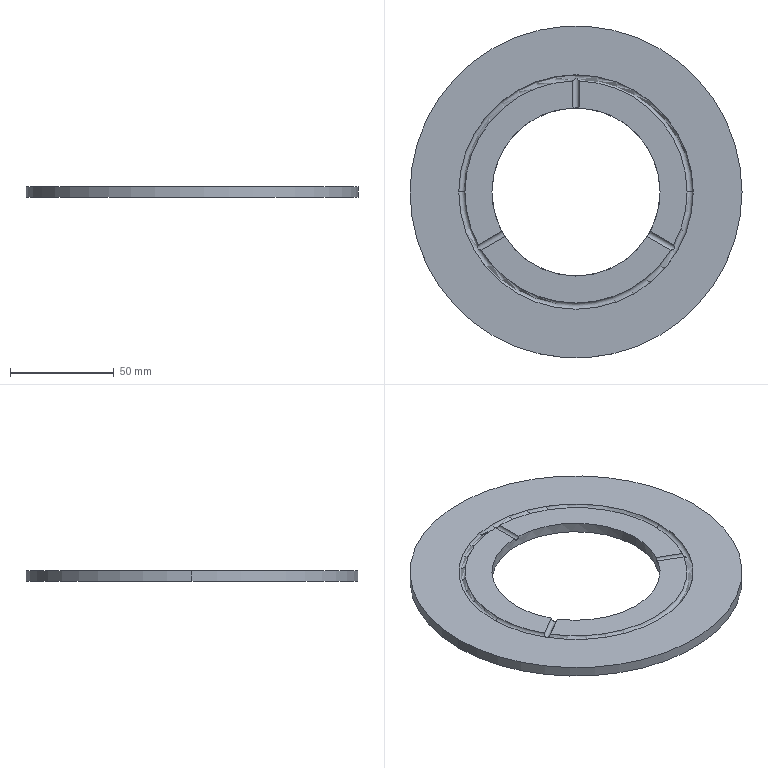Part | SolidWorks | features CirPattern 1, Extrusion 1, ICE 1, SweepCut 1 | 1 solid | 15 faces | box 160 x 160 x 5 mm | volume 73404 mm3 | cylinder 8 | plane 5 | torus 2 | commonest cylinder face diameters 3 x4 81 x2 160 x2
STEP:
#1=CARTESIAN_POINT('',(0.,55.,3.5));
#2=VERTEX_POINT('',#1);
#3=CARTESIAN_POINT('',(1.5,53.479,5.));
#4=VERTEX_POINT('',#3);
#5=CARTESIAN_POINT('',(0.,55.,3.5));
#6=CARTESIAN_POINT('',(0.08396,54.916,3.5));
#7=CARTESIAN_POINT('',(0.1693,54.83,3.507));
#8=CARTESIAN_POINT('',(0.3359,54.663,3.536));
#9=CARTESIAN_POINT('',(0.4182,54.58,3.557));
#10=CARTESIAN_POINT('',(0.6622,54.334,3.643));
#11=CARTESIAN_POINT('',(0.8218,54.172,3.731));
#12=CARTESIAN_POINT('',(1.11,53.879,3.974));
#13=CARTESIAN_POINT('',(1.242,53.744,4.131));
#14=CARTESIAN_POINT('',(1.39,53.592,4.425));
#15=CARTESIAN_POINT('',(1.43,53.551,4.531));
#16=CARTESIAN_POINT('',(1.485,53.494,4.758));
#17=CARTESIAN_POINT('',(1.5,53.479,4.878));
#18=CARTESIAN_POINT('',(1.5,53.479,5.));
#19=B_SPLINE_CURVE_WITH_KNOTS('',3,(#5,#6,#7,#8,#9,#10,#11,#12,#13,#14,#15,#16,#17,#18),.UNSPECIFIED.,.F.,.F.,(4,2,2,2,2,2,4),(-0.000007746,0.0003485,0.0007047,0.001417,0.00213,0.002486,0.002842),.UNSPECIFIED.);
#20=EDGE_CURVE('',#2,#4,#19,.T.);
#21=ORIENTED_EDGE('',*,*,#20,.F.);
#22=CARTESIAN_POINT('',(0.,40.5,3.5));
#23=VERTEX_POINT('',#22);
#24=CARTESIAN_POINT('',(0.,55.,3.5));
#25=DIRECTION('',(0.,-1.,0.));
#26=VECTOR('',#25,1000.);
#27=LINE('',#24,#26);
#28=EDGE_CURVE('',#2,#23,#27,.T.);
#29=ORIENTED_EDGE('',*,*,#28,.T.);
#30=CARTESIAN_POINT('',(1.5,40.472,5.));
#31=VERTEX_POINT('',#30);
#32=CARTESIAN_POINT('',(1.5,40.472,5.));
#33=CARTESIAN_POINT('',(1.5,40.472,4.901));
#34=CARTESIAN_POINT('',(1.49,40.473,4.803));
#35=CARTESIAN_POINT('',(1.452,40.474,4.612));
#36=CARTESIAN_POINT('',(1.423,40.475,4.516));
#37=CARTESIAN_POINT('',(1.348,40.478,4.335));
#38=CARTESIAN_POINT('',(1.302,40.479,4.248));
#39=CARTESIAN_POINT('',(1.193,40.482,4.085));
#40=CARTESIAN_POINT('',(1.13,40.484,4.008));
#41=CARTESIAN_POINT('',(0.9218,40.49,3.801));
#42=CARTESIAN_POINT('',(0.7544,40.493,3.689));
#43=CARTESIAN_POINT('',(0.3932,40.498,3.539));
#44=CARTESIAN_POINT('',(0.1957,40.5,3.5));
#45=CARTESIAN_POINT('',(0.,40.5,3.5));
#46=B_SPLINE_CURVE_WITH_KNOTS('',3,(#32,#33,#34,#35,#36,#37,#38,#39,#40,#41,#42,#43,#44,#45),.UNSPECIFIED.,.F.,.F.,(4,2,2,2,2,2,4),(0.,0.0002932,0.0005864,0.0008796,0.001173,0.001759,0.002346),.UNSPECIFIED.);
#47=EDGE_CURVE('',#31,#23,#46,.T.);
#48=ORIENTED_EDGE('',*,*,#47,.F.);
#49=CARTESIAN_POINT('',(1.5,55.,5.));
#50=DIRECTION('',(0.,-1.,0.));
#51=VECTOR('',#50,1000.);
#52=LINE('',#49,#51);
#53=EDGE_CURVE('',#4,#31,#52,.T.);
#54=ORIENTED_EDGE('',*,*,#53,.F.);
#55=EDGE_LOOP('',(#21,#29,#48,#54));
#56=FACE_OUTER_BOUND('',#55,.T.);
#57=CARTESIAN_POINT('',(0.,55.,5.));
#58=DIRECTION('',(0.,-1.,0.));
#59=DIRECTION('',(0.,0.,-1.));
#60=AXIS2_PLACEMENT_3D('',#57,#58,#59);
#61=CYLINDRICAL_SURFACE('',#60,1.5);
#62=ADVANCED_FACE('',(#56),#61,.F.);
#63=CARTESIAN_POINT('',(80.,0.,5.));
#64=VERTEX_POINT('',#63);
#65=CARTESIAN_POINT('',(-80.,0.,5.));
#66=VERTEX_POINT('',#65);
#67=CARTESIAN_POINT('',(0.,0.,5.));
#68=DIRECTION('',(0.,0.,1.));
#69=DIRECTION('',(1.,0.,0.));
#70=AXIS2_PLACEMENT_3D('',#67,#68,#69);
#71=CIRCLE('',#70,80.);
#72=EDGE_CURVE('',#64,#66,#71,.T.);
#73=ORIENTED_EDGE('',*,*,#72,.F.);
#74=CARTESIAN_POINT('',(80.,0.,0.));
#75=VERTEX_POINT('',#74);
#76=CARTESIAN_POINT('',(80.,0.,5.));
#77=DIRECTION('',(0.,0.,-1.));
#78=VECTOR('',#77,1000.);
#79=LINE('',#76,#78);
#80=EDGE_CURVE('',#64,#75,#79,.T.);
#81=ORIENTED_EDGE('',*,*,#80,.T.);
#82=CARTESIAN_POINT('',(-80.,0.,0.));
#83=VERTEX_POINT('',#82);
#84=CARTESIAN_POINT('',(0.,0.,0.));
#85=DIRECTION('',(0.,0.,1.));
#86=DIRECTION('',(1.,0.,0.));
#87=AXIS2_PLACEMENT_3D('',#84,#85,#86);
#88=CIRCLE('',#87,80.);
#89=EDGE_CURVE('',#75,#83,#88,.T.);
#90=ORIENTED_EDGE('',*,*,#89,.T.);
#91=CARTESIAN_POINT('',(-80.,0.,5.));
#92=DIRECTION('',(0.,0.,-1.));
#93=VECTOR('',#92,1000.);
#94=LINE('',#91,#93);
#95=EDGE_CURVE('',#66,#83,#94,.T.);
#96=ORIENTED_EDGE('',*,*,#95,.F.);
#97=EDGE_LOOP('',(#73,#81,#90,#96));
#98=FACE_OUTER_BOUND('',#97,.T.);
#99=CARTESIAN_POINT('',(0.,0.,5.));
#100=DIRECTION('',(0.,0.,-1.));
#101=DIRECTION('',(-1.,0.,0.));
#102=AXIS2_PLACEMENT_3D('',#99,#100,#101);
#103=CYLINDRICAL_SURFACE('',#102,80.);
#104=ADVANCED_FACE('',(#98),#103,.T.);
#105=CARTESIAN_POINT('',(-53.5,0.,5.));
#106=VERTEX_POINT('',#105);
#107=CARTESIAN_POINT('',(-47.064,-25.44,5.));
#108=VERTEX_POINT('',#107);
#109=CARTESIAN_POINT('',(0.,0.,5.));
#110=DIRECTION('',(0.,0.,1.));
#111=DIRECTION('',(-1.,0.,0.));
#112=AXIS2_PLACEMENT_3D('',#109,#110,#111);
#113=CIRCLE('',#112,53.5);
#114=EDGE_CURVE('',#106,#108,#113,.T.);
#115=ORIENTED_EDGE('',*,*,#114,.F.);
#116=CARTESIAN_POINT('',(-56.5,0.,5.));
#117=VERTEX_POINT('',#116);
#118=CARTESIAN_POINT('',(-55.,0.,5.));
#119=DIRECTION('',(0.,1.,0.));
#120=DIRECTION('',(-1.,0.,0.));
#121=AXIS2_PLACEMENT_3D('',#118,#119,#120);
#122=CIRCLE('',#121,1.5);
#123=EDGE_CURVE('',#106,#117,#122,.T.);
#124=ORIENTED_EDGE('',*,*,#123,.T.);
#125=CARTESIAN_POINT('',(56.5,0.,5.));
#126=VERTEX_POINT('',#125);
#127=CARTESIAN_POINT('',(0.,0.,5.));
#128=DIRECTION('',(0.,0.,-1.));
#129=DIRECTION('',(1.,0.,0.));
#130=AXIS2_PLACEMENT_3D('',#127,#128,#129);
#131=CIRCLE('',#130,56.5);
#132=EDGE_CURVE('',#126,#117,#131,.T.);
#133=ORIENTED_EDGE('',*,*,#132,.F.);
#134=CARTESIAN_POINT('',(53.5,0.,5.));
#135=VERTEX_POINT('',#134);
#136=CARTESIAN_POINT('',(55.,0.,5.));
#137=DIRECTION('',(0.,-1.,0.));
#138=DIRECTION('',(0.,0.,-1.));
#139=AXIS2_PLACEMENT_3D('',#136,#137,#138);
#140=CIRCLE('',#139,1.5);
#141=EDGE_CURVE('',#135,#126,#140,.T.);
#142=ORIENTED_EDGE('',*,*,#141,.F.);
#143=CARTESIAN_POINT('',(47.064,-25.44,5.));
#144=VERTEX_POINT('',#143);
#145=CARTESIAN_POINT('',(0.,0.,5.));
#146=DIRECTION('',(0.,0.,1.));
#147=DIRECTION('',(-1.,0.,0.));
#148=AXIS2_PLACEMENT_3D('',#145,#146,#147);
#149=CIRCLE('',#148,53.5);
#150=EDGE_CURVE('',#144,#135,#149,.T.);
#151=ORIENTED_EDGE('',*,*,#150,.F.);
#152=CARTESIAN_POINT('',(47.631,-27.5,3.5));
#153=VERTEX_POINT('',#152);
#154=CARTESIAN_POINT('',(47.064,-25.44,5.));
#155=CARTESIAN_POINT('',(47.064,-25.44,4.757));
#156=CARTESIAN_POINT('',(47.088,-25.524,4.524));
#157=CARTESIAN_POINT('',(47.164,-25.794,4.133));
#158=CARTESIAN_POINT('',(47.215,-25.975,3.976));
#159=CARTESIAN_POINT('',(47.325,-26.373,3.731));
#160=CARTESIAN_POINT('',(47.384,-26.587,3.645));
#161=CARTESIAN_POINT('',(47.507,-27.038,3.528));
#162=CARTESIAN_POINT('',(47.57,-27.269,3.5));
#163=CARTESIAN_POINT('',(47.631,-27.5,3.5));
#164=B_SPLINE_CURVE_WITH_KNOTS('',3,(#154,#155,#156,#157,#158,#159,#160,#161,#162,#163),.UNSPECIFIED.,.F.,.F.,(4,2,2,2,4),(0.000000196,0.0007165,0.001433,0.002149,0.002865),.UNSPECIFIED.);
#165=EDGE_CURVE('',#144,#153,#164,.T.);
#166=ORIENTED_EDGE('',*,*,#165,.T.);
#167=CARTESIAN_POINT('',(45.564,-28.039,5.));
#168=VERTEX_POINT('',#167);
#169=CARTESIAN_POINT('',(47.631,-27.5,3.5));
#170=CARTESIAN_POINT('',(47.517,-27.531,3.5));
#171=CARTESIAN_POINT('',(47.4,-27.562,3.507));
#172=CARTESIAN_POINT('',(47.172,-27.622,3.536));
#173=CARTESIAN_POINT('',(47.059,-27.652,3.557));
#174=CARTESIAN_POINT('',(46.724,-27.74,3.643));
#175=CARTESIAN_POINT('',(46.504,-27.798,3.731));
#176=CARTESIAN_POINT('',(46.105,-27.901,3.974));
#177=CARTESIAN_POINT('',(45.923,-27.947,4.131));
#178=CARTESIAN_POINT('',(45.718,-28.,4.425));
#179=CARTESIAN_POINT('',(45.662,-28.014,4.531));
#180=CARTESIAN_POINT('',(45.585,-28.033,4.758));
#181=CARTESIAN_POINT('',(45.564,-28.039,4.878));
#182=CARTESIAN_POINT('',(45.564,-28.039,5.));
#183=B_SPLINE_CURVE_WITH_KNOTS('',3,(#169,#170,#171,#172,#173,#174,#175,#176,#177,#178,#179,#180,#181,#182),.UNSPECIFIED.,.F.,.F.,(4,2,2,2,2,2,4),(-0.000007746,0.0003485,0.0007047,0.001417,0.00213,0.002486,0.002842),.UNSPECIFIED.);
#184=EDGE_CURVE('',#153,#168,#183,.T.);
#185=ORIENTED_EDGE('',*,*,#184,.T.);
#186=CARTESIAN_POINT('',(-45.564,-28.039,5.));
#187=VERTEX_POINT('',#186);
#188=CARTESIAN_POINT('',(0.,0.,5.));
#189=DIRECTION('',(0.,0.,1.));
#190=DIRECTION('',(-1.,0.,0.));
#191=AXIS2_PLACEMENT_3D('',#188,#189,#190);
#192=CIRCLE('',#191,53.5);
#193=EDGE_CURVE('',#187,#168,#192,.T.);
#194=ORIENTED_EDGE('',*,*,#193,.F.);
#195=CARTESIAN_POINT('',(-47.631,-27.5,3.5));
#196=VERTEX_POINT('',#195);
#197=CARTESIAN_POINT('',(-45.564,-28.039,5.));
#198=CARTESIAN_POINT('',(-45.564,-28.039,4.757));
#199=CARTESIAN_POINT('',(-45.649,-28.017,4.524));
#200=CARTESIAN_POINT('',(-45.921,-27.948,4.133));
#201=CARTESIAN_POINT('',(-46.102,-27.901,3.976));
#202=CARTESIAN_POINT('',(-46.503,-27.798,3.731));
#203=CARTESIAN_POINT('',(-46.717,-27.742,3.645));
#204=CARTESIAN_POINT('',(-47.169,-27.623,3.528));
#205=CARTESIAN_POINT('',(-47.401,-27.562,3.5));
#206=CARTESIAN_POINT('',(-47.631,-27.5,3.5));
#207=B_SPLINE_CURVE_WITH_KNOTS('',3,(#197,#198,#199,#200,#201,#202,#203,#204,#205,#206),.UNSPECIFIED.,.F.,.F.,(4,2,2,2,4),(0.000000196,0.0007165,0.001433,0.002149,0.002865),.UNSPECIFIED.);
#208=EDGE_CURVE('',#187,#196,#207,.T.);
#209=ORIENTED_EDGE('',*,*,#208,.T.);
#210=CARTESIAN_POINT('',(-47.631,-27.5,3.5));
#211=CARTESIAN_POINT('',(-47.601,-27.385,3.5));
#212=CARTESIAN_POINT('',(-47.569,-27.269,3.507));
#213=CARTESIAN_POINT('',(-47.508,-27.041,3.536));
#214=CARTESIAN_POINT('',(-47.477,-26.928,3.557));
#215=CARTESIAN_POINT('',(-47.386,-26.594,3.643));
#216=CARTESIAN_POINT('',(-47.325,-26.374,3.731));
#217=CARTESIAN_POINT('',(-47.215,-25.978,3.974));
#218=CARTESIAN_POINT('',(-47.165,-25.797,4.131));
#219=CARTESIAN_POINT('',(-47.107,-25.593,4.425));
#220=CARTESIAN_POINT('',(-47.092,-25.538,4.531));
#221=CARTESIAN_POINT('',(-47.07,-25.461,4.758));
#222=CARTESIAN_POINT('',(-47.064,-25.44,4.878));
#223=CARTESIAN_POINT('',(-47.064,-25.44,5.));
#224=B_SPLINE_CURVE_WITH_KNOTS('',3,(#210,#211,#212,#213,#214,#215,#216,#217,#218,#219,#220,#221,#222,#223),.UNSPECIFIED.,.F.,.F.,(4,2,2,2,2,2,4),(-0.000007746,0.0003485,0.0007047,0.001417,0.00213,0.002486,0.002842),.UNSPECIFIED.);
#225=EDGE_CURVE('',#196,#108,#224,.T.);
#226=ORIENTED_EDGE('',*,*,#225,.T.);
#227=EDGE_LOOP('',(#115,#124,#133,#142,#151,#166,#185,#194,#209,#226));
#228=FACE_OUTER_BOUND('',#227,.T.);
#229=CARTESIAN_POINT('',(0.,0.,5.));
#230=DIRECTION('',(0.,0.,1.));
#231=DIRECTION('',(1.,0.,0.));
#232=AXIS2_PLACEMENT_3D('',#229,#230,#231);
#233=TOROIDAL_SURFACE('',#232,55.,1.5);
#234=ADVANCED_FACE('',(#228),#233,.F.);
#235=CARTESIAN_POINT('',(35.8,-18.937,5.));
#236=VERTEX_POINT('',#235);
#237=CARTESIAN_POINT('',(40.5,0.,5.));
#238=VERTEX_POINT('',#237);
#239=CARTESIAN_POINT('',(0.,0.,5.));
#240=DIRECTION('',(0.,0.,1.));
#241=DIRECTION('',(1.,0.,0.));
#242=AXIS2_PLACEMENT_3D('',#239,#240,#241);
#243=CIRCLE('',#242,40.5);
#244=EDGE_CURVE('',#236,#238,#243,.T.);
#245=ORIENTED_EDGE('',*,*,#244,.T.);
#246=CARTESIAN_POINT('',(40.5,0.,0.));
#247=VERTEX_POINT('',#246);
#248=CARTESIAN_POINT('',(40.5,0.,5.));
#249=DIRECTION('',(0.,0.,-1.));
#250=VECTOR('',#249,1000.);
#251=LINE('',#248,#250);
#252=EDGE_CURVE('',#238,#247,#251,.T.);
#253=ORIENTED_EDGE('',*,*,#252,.T.);
#254=CARTESIAN_POINT('',(-40.5,0.,0.));
#255=VERTEX_POINT('',#254);
#256=CARTESIAN_POINT('',(0.,0.,0.));
#257=DIRECTION('',(0.,0.,1.));
#258=DIRECTION('',(1.,0.,0.));
#259=AXIS2_PLACEMENT_3D('',#256,#257,#258);
#260=CIRCLE('',#259,40.5);
#261=EDGE_CURVE('',#255,#247,#260,.T.);
#262=ORIENTED_EDGE('',*,*,#261,.F.);
#263=CARTESIAN_POINT('',(-40.5,0.,5.));
#264=VERTEX_POINT('',#263);
#265=CARTESIAN_POINT('',(-40.5,0.,5.));
#266=DIRECTION('',(0.,0.,-1.));
#267=VECTOR('',#266,1000.);
#268=LINE('',#265,#267);
#269=EDGE_CURVE('',#264,#255,#268,.T.);
#270=ORIENTED_EDGE('',*,*,#269,.F.);
#271=CARTESIAN_POINT('',(-35.8,-18.937,5.));
#272=VERTEX_POINT('',#271);
#273=CARTESIAN_POINT('',(0.,0.,5.));
#274=DIRECTION('',(0.,0.,1.));
#275=DIRECTION('',(1.,0.,0.));
#276=AXIS2_PLACEMENT_3D('',#273,#274,#275);
#277=CIRCLE('',#276,40.5);
#278=EDGE_CURVE('',#264,#272,#277,.T.);
#279=ORIENTED_EDGE('',*,*,#278,.T.);
#280=CARTESIAN_POINT('',(-34.3,-21.535,5.));
#281=VERTEX_POINT('',#280);
#282=CARTESIAN_POINT('',(-35.8,-18.937,5.));
#283=CARTESIAN_POINT('',(-35.8,-18.937,4.901));
#284=CARTESIAN_POINT('',(-35.795,-18.946,4.803));
#285=CARTESIAN_POINT('',(-35.778,-18.979,4.612));
#286=CARTESIAN_POINT('',(-35.764,-19.005,4.516));
#287=CARTESIAN_POINT('',(-35.729,-19.071,4.335));
#288=CARTESIAN_POINT('',(-35.707,-19.112,4.249));
#289=CARTESIAN_POINT('',(-35.655,-19.208,4.086));
#290=CARTESIAN_POINT('',(-35.625,-19.264,4.008));
#291=CARTESIAN_POINT('',(-35.526,-19.446,3.801));
#292=CARTESIAN_POINT('',(-35.446,-19.593,3.689));
#293=CARTESIAN_POINT('',(-35.27,-19.908,3.539));
#294=CARTESIAN_POINT('',(-35.172,-20.08,3.5));
#295=CARTESIAN_POINT('',(-35.025,-20.334,3.5));
#296=CARTESIAN_POINT('',(-34.975,-20.42,3.51));
#297=CARTESIAN_POINT('',(-34.878,-20.586,3.548));
#298=CARTESIAN_POINT('',(-34.83,-20.667,3.576));
#299=CARTESIAN_POINT('',(-34.737,-20.823,3.651));
#300=CARTESIAN_POINT('',(-34.692,-20.898,3.698));
#301=CARTESIAN_POINT('',(-34.608,-21.037,3.807));
#302=CARTESIAN_POINT('',(-34.568,-21.102,3.869));
#303=CARTESIAN_POINT('',(-34.459,-21.281,4.079));
#304=CARTESIAN_POINT('',(-34.4,-21.374,4.244));
#305=CARTESIAN_POINT('',(-34.341,-21.47,4.517));
#306=CARTESIAN_POINT('',(-34.326,-21.494,4.61));
#307=CARTESIAN_POINT('',(-34.305,-21.527,4.803));
#308=CARTESIAN_POINT('',(-34.3,-21.535,4.902));
#309=CARTESIAN_POINT('',(-34.3,-21.535,5.));
#310=B_SPLINE_CURVE_WITH_KNOTS('',3,(#282,#283,#284,#285,#286,#287,#288,#289,#290,#291,#292,#293,#294,#295,#296,#297,#298,#299,#300,#301,#302,#303,#304,#305,#306,#307,#308,#309),.UNSPECIFIED.,.F.,.F.,(4,2,2,2,2,2,2,2,2,2,2,2,2,4),(0.,0.0002931,0.0005863,0.0008794,0.001173,0.001759,0.002345,0.002638,0.002931,0.003224,0.003518,0.004104,0.004397,0.00469),.UNSPECIFIED.);
#311=EDGE_CURVE('',#272,#281,#310,.T.);
#312=ORIENTED_EDGE('',*,*,#311,.T.);
#313=CARTESIAN_POINT('',(34.3,-21.535,5.));
#314=VERTEX_POINT('',#313);
#315=CARTESIAN_POINT('',(0.,0.,5.));
#316=DIRECTION('',(0.,0.,1.));
#317=DIRECTION('',(1.,0.,0.));
#318=AXIS2_PLACEMENT_3D('',#315,#316,#317);
#319=CIRCLE('',#318,40.5);
#320=EDGE_CURVE('',#281,#314,#319,.T.);
#321=ORIENTED_EDGE('',*,*,#320,.T.);
#322=CARTESIAN_POINT('',(34.3,-21.535,5.));
#323=CARTESIAN_POINT('',(34.3,-21.535,4.901));
#324=CARTESIAN_POINT('',(34.305,-21.527,4.803));
#325=CARTESIAN_POINT('',(34.325,-21.495,4.612));
#326=CARTESIAN_POINT('',(34.341,-21.47,4.516));
#327=CARTESIAN_POINT('',(34.381,-21.406,4.335));
#328=CARTESIAN_POINT('',(34.405,-21.367,4.249));
#329=CARTESIAN_POINT('',(34.462,-21.274,4.086));
#330=CARTESIAN_POINT('',(34.496,-21.22,4.008));
#331=CARTESIAN_POINT('',(34.604,-21.043,3.801));
#332=CARTESIAN_POINT('',(34.691,-20.9,3.689));
#333=CARTESIAN_POINT('',(34.876,-20.59,3.539));
#334=CARTESIAN_POINT('',(34.976,-20.42,3.5));
#335=CARTESIAN_POINT('',(35.123,-20.166,3.5));
#336=CARTESIAN_POINT('',(35.172,-20.079,3.51));
#337=CARTESIAN_POINT('',(35.267,-19.912,3.548));
#338=CARTESIAN_POINT('',(35.313,-19.831,3.576));
#339=CARTESIAN_POINT('',(35.402,-19.672,3.651));
#340=CARTESIAN_POINT('',(35.444,-19.595,3.698));
#341=CARTESIAN_POINT('',(35.522,-19.453,3.807));
#342=CARTESIAN_POINT('',(35.559,-19.386,3.869));
#343=CARTESIAN_POINT('',(35.659,-19.202,4.079));
#344=CARTESIAN_POINT('',(35.711,-19.104,4.244));
#345=CARTESIAN_POINT('',(35.764,-19.005,4.517));
#346=CARTESIAN_POINT('',(35.777,-18.98,4.61));
#347=CARTESIAN_POINT('',(35.795,-18.946,4.803));
#348=CARTESIAN_POINT('',(35.8,-18.937,4.902));
#349=CARTESIAN_POINT('',(35.8,-18.937,5.));
#350=B_SPLINE_CURVE_WITH_KNOTS('',3,(#322,#323,#324,#325,#326,#327,#328,#329,#330,#331,#332,#333,#334,#335,#336,#337,#338,#339,#340,#341,#342,#343,#344,#345,#346,#347,#348,#349),.UNSPECIFIED.,.F.,.F.,(4,2,2,2,2,2,2,2,2,2,2,2,2,4),(0.,0.0002931,0.0005863,0.0008794,0.001173,0.001759,0.002345,0.002638,0.002931,0.003224,0.003518,0.004104,0.004397,0.00469),.UNSPECIFIED.);
#351=EDGE_CURVE('',#314,#236,#350,.T.);
#352=ORIENTED_EDGE('',*,*,#351,.T.);
#353=EDGE_LOOP('',(#245,#253,#262,#270,#279,#312,#321,#352));
#354=FACE_OUTER_BOUND('',#353,.T.);
#355=CARTESIAN_POINT('',(0.,0.,5.));
#356=DIRECTION('',(0.,0.,-1.));
#357=DIRECTION('',(-1.,0.,0.));
#358=AXIS2_PLACEMENT_3D('',#355,#356,#357);
#359=CYLINDRICAL_SURFACE('',#358,40.5);
#360=ADVANCED_FACE('',(#354),#359,.F.);
#361=ORIENTED_EDGE('',*,*,#244,.F.);
#362=CARTESIAN_POINT('',(48.381,-26.201,5.));
#363=DIRECTION('',(0.866,-0.5,0.));
#364=VECTOR('',#363,1000.);
#365=LINE('',#362,#364);
#366=EDGE_CURVE('',#236,#144,#365,.T.);
#367=ORIENTED_EDGE('',*,*,#366,.T.);
#368=ORIENTED_EDGE('',*,*,#150,.T.);
#369=CARTESIAN_POINT('',(0.,0.,5.));
#370=DIRECTION('',(0.,0.,1.));
#371=DIRECTION('',(-1.,0.,0.));
#372=AXIS2_PLACEMENT_3D('',#369,#370,#371);
#373=CIRCLE('',#372,53.5);
#374=EDGE_CURVE('',#135,#4,#373,.T.);
#375=ORIENTED_EDGE('',*,*,#374,.T.);
#376=ORIENTED_EDGE('',*,*,#53,.T.);
#377=CARTESIAN_POINT('',(0.,0.,5.));
#378=DIRECTION('',(0.,0.,1.));
#379=DIRECTION('',(1.,0.,0.));
#380=AXIS2_PLACEMENT_3D('',#377,#378,#379);
#381=CIRCLE('',#380,40.5);
#382=EDGE_CURVE('',#238,#31,#381,.T.);
#383=ORIENTED_EDGE('',*,*,#382,.F.);
#384=EDGE_LOOP('',(#361,#367,#368,#375,#376,#383));
#385=FACE_OUTER_BOUND('',#384,.T.);
#386=CARTESIAN_POINT('',(0.,0.,5.));
#387=DIRECTION('',(0.,0.,1.));
#388=DIRECTION('',(1.,0.,0.));
#389=AXIS2_PLACEMENT_3D('',#386,#387,#388);
#390=PLANE('',#389);
#391=ADVANCED_FACE('',(#385),#390,.T.);
#392=ORIENTED_EDGE('',*,*,#193,.T.);
#393=CARTESIAN_POINT('',(46.881,-28.799,5.));
#394=DIRECTION('',(-0.866,0.5,0.));
#395=VECTOR('',#394,1000.);
#396=LINE('',#393,#395);
#397=EDGE_CURVE('',#168,#314,#396,.T.);
#398=ORIENTED_EDGE('',*,*,#397,.T.);
#399=ORIENTED_EDGE('',*,*,#320,.F.);
#400=CARTESIAN_POINT('',(-46.881,-28.799,5.));
#401=DIRECTION('',(-0.866,-0.5,0.));
#402=VECTOR('',#401,1000.);
#403=LINE('',#400,#402);
#404=EDGE_CURVE('',#281,#187,#403,.T.);
#405=ORIENTED_EDGE('',*,*,#404,.T.);
#406=EDGE_LOOP('',(#392,#398,#399,#405));
#407=FACE_OUTER_BOUND('',#406,.T.);
#408=CARTESIAN_POINT('',(0.,0.,5.));
#409=DIRECTION('',(0.,0.,1.));
#410=DIRECTION('',(1.,0.,0.));
#411=AXIS2_PLACEMENT_3D('',#408,#409,#410);
#412=PLANE('',#411);
#413=ADVANCED_FACE('',(#407),#412,.T.);
#414=CARTESIAN_POINT('',(-1.5,53.479,5.));
#415=VERTEX_POINT('',#414);
#416=CARTESIAN_POINT('',(0.,0.,5.));
#417=DIRECTION('',(0.,0.,1.));
#418=DIRECTION('',(-1.,0.,0.));
#419=AXIS2_PLACEMENT_3D('',#416,#417,#418);
#420=CIRCLE('',#419,53.5);
#421=EDGE_CURVE('',#415,#106,#420,.T.);
#422=ORIENTED_EDGE('',*,*,#421,.T.);
#423=ORIENTED_EDGE('',*,*,#114,.T.);
#424=CARTESIAN_POINT('',(-48.381,-26.201,5.));
#425=DIRECTION('',(0.866,0.5,0.));
#426=VECTOR('',#425,1000.);
#427=LINE('',#424,#426);
#428=EDGE_CURVE('',#108,#272,#427,.T.);
#429=ORIENTED_EDGE('',*,*,#428,.T.);
#430=ORIENTED_EDGE('',*,*,#278,.F.);
#431=CARTESIAN_POINT('',(-1.5,40.472,5.));
#432=VERTEX_POINT('',#431);
#433=CARTESIAN_POINT('',(0.,0.,5.));
#434=DIRECTION('',(0.,0.,1.));
#435=DIRECTION('',(1.,0.,0.));
#436=AXIS2_PLACEMENT_3D('',#433,#434,#435);
#437=CIRCLE('',#436,40.5);
#438=EDGE_CURVE('',#432,#264,#437,.T.);
#439=ORIENTED_EDGE('',*,*,#438,.F.);
#440=CARTESIAN_POINT('',(-1.5,55.,5.));
#441=DIRECTION('',(0.,1.,0.));
#442=VECTOR('',#441,1000.);
#443=LINE('',#440,#442);
#444=EDGE_CURVE('',#432,#415,#443,.T.);
#445=ORIENTED_EDGE('',*,*,#444,.T.);
#446=EDGE_LOOP('',(#422,#423,#429,#430,#439,#445));
#447=FACE_OUTER_BOUND('',#446,.T.);
#448=CARTESIAN_POINT('',(0.,0.,5.));
#449=DIRECTION('',(0.,0.,1.));
#450=DIRECTION('',(1.,0.,0.));
#451=AXIS2_PLACEMENT_3D('',#448,#449,#450);
#452=PLANE('',#451);
#453=ADVANCED_FACE('',(#447),#452,.T.);
#454=ORIENTED_EDGE('',*,*,#252,.F.);
#455=ORIENTED_EDGE('',*,*,#382,.T.);
#456=ORIENTED_EDGE('',*,*,#47,.T.);
#457=CARTESIAN_POINT('',(0.,40.5,3.5));
#458=CARTESIAN_POINT('',(-0.09778,40.5,3.5));
#459=CARTESIAN_POINT('',(-0.1971,40.5,3.51));
#460=CARTESIAN_POINT('',(-0.3894,40.498,3.548));
#461=CARTESIAN_POINT('',(-0.4828,40.497,3.576));
#462=CARTESIAN_POINT('',(-0.6643,40.495,3.652));
#463=CARTESIAN_POINT('',(-0.7521,40.493,3.698));
#464=CARTESIAN_POINT('',(-0.9145,40.49,3.807));
#465=CARTESIAN_POINT('',(-0.9903,40.488,3.869));
#466=CARTESIAN_POINT('',(-1.2,40.482,4.079));
#467=CARTESIAN_POINT('',(-1.31,40.479,4.244));
#468=CARTESIAN_POINT('',(-1.461,40.474,4.607));
#469=CARTESIAN_POINT('',(-1.5,40.472,4.802));
#470=CARTESIAN_POINT('',(-1.5,40.472,5.));
#471=B_SPLINE_CURVE_WITH_KNOTS('',3,(#457,#458,#459,#460,#461,#462,#463,#464,#465,#466,#467,#468,#469,#470),.UNSPECIFIED.,.F.,.F.,(4,2,2,2,2,2,4),(0.002346,0.002639,0.002931,0.003224,0.003517,0.004103,0.004689),.UNSPECIFIED.);
#472=EDGE_CURVE('',#23,#432,#471,.T.);
#473=ORIENTED_EDGE('',*,*,#472,.T.);
#474=ORIENTED_EDGE('',*,*,#438,.T.);
#475=ORIENTED_EDGE('',*,*,#269,.T.);
#476=CARTESIAN_POINT('',(0.,0.,0.));
#477=DIRECTION('',(0.,0.,1.));
#478=DIRECTION('',(1.,0.,0.));
#479=AXIS2_PLACEMENT_3D('',#476,#477,#478);
#480=CIRCLE('',#479,40.5);
#481=EDGE_CURVE('',#247,#255,#480,.T.);
#482=ORIENTED_EDGE('',*,*,#481,.F.);
#483=EDGE_LOOP('',(#454,#455,#456,#473,#474,#475,#482));
#484=FACE_OUTER_BOUND('',#483,.T.);
#485=CARTESIAN_POINT('',(0.,0.,5.));
#486=DIRECTION('',(0.,0.,-1.));
#487=DIRECTION('',(-1.,0.,0.));
#488=AXIS2_PLACEMENT_3D('',#485,#486,#487);
#489=CYLINDRICAL_SURFACE('',#488,40.5);
#490=ADVANCED_FACE('',(#484),#489,.F.);
#491=ORIENTED_EDGE('',*,*,#123,.F.);
#492=ORIENTED_EDGE('',*,*,#421,.F.);
#493=CARTESIAN_POINT('',(-1.5,53.479,5.));
#494=CARTESIAN_POINT('',(-1.5,53.479,4.757));
#495=CARTESIAN_POINT('',(-1.439,53.542,4.524));
#496=CARTESIAN_POINT('',(-1.243,53.742,4.133));
#497=CARTESIAN_POINT('',(-1.112,53.877,3.976));
#498=CARTESIAN_POINT('',(-0.8225,54.171,3.731));
#499=CARTESIAN_POINT('',(-0.6666,54.33,3.645));
#500=CARTESIAN_POINT('',(-0.3377,54.661,3.528));
#501=CARTESIAN_POINT('',(-0.1688,54.831,3.5));
#502=CARTESIAN_POINT('',(0.,55.,3.5));
#503=B_SPLINE_CURVE_WITH_KNOTS('',3,(#493,#494,#495,#496,#497,#498,#499,#500,#501,#502),.UNSPECIFIED.,.F.,.F.,(4,2,2,2,4),(0.000000196,0.0007165,0.001433,0.002149,0.002865),.UNSPECIFIED.);
#504=EDGE_CURVE('',#415,#2,#503,.T.);
#505=ORIENTED_EDGE('',*,*,#504,.T.);
#506=ORIENTED_EDGE('',*,*,#20,.T.);
#507=ORIENTED_EDGE('',*,*,#374,.F.);
#508=ORIENTED_EDGE('',*,*,#141,.T.);
#509=CARTESIAN_POINT('',(0.,0.,5.));
#510=DIRECTION('',(0.,0.,-1.));
#511=DIRECTION('',(1.,0.,0.));
#512=AXIS2_PLACEMENT_3D('',#509,#510,#511);
#513=CIRCLE('',#512,56.5);
#514=EDGE_CURVE('',#117,#126,#513,.T.);
#515=ORIENTED_EDGE('',*,*,#514,.F.);
#516=EDGE_LOOP('',(#491,#492,#505,#506,#507,#508,#515));
#517=FACE_OUTER_BOUND('',#516,.T.);
#518=CARTESIAN_POINT('',(0.,0.,5.));
#519=DIRECTION('',(0.,0.,1.));
#520=DIRECTION('',(1.,0.,0.));
#521=AXIS2_PLACEMENT_3D('',#518,#519,#520);
#522=TOROIDAL_SURFACE('',#521,55.,1.5);
#523=ADVANCED_FACE('',(#517),#522,.F.);
#524=CARTESIAN_POINT('',(0.,0.,5.));
#525=DIRECTION('',(0.,0.,1.));
#526=DIRECTION('',(1.,0.,0.));
#527=AXIS2_PLACEMENT_3D('',#524,#525,#526);
#528=CIRCLE('',#527,80.);
#529=EDGE_CURVE('',#66,#64,#528,.T.);
#530=ORIENTED_EDGE('',*,*,#529,.T.);
#531=ORIENTED_EDGE('',*,*,#72,.T.);
#532=EDGE_LOOP('',(#530,#531));
#533=FACE_OUTER_BOUND('',#532,.T.);
#534=ORIENTED_EDGE('',*,*,#132,.T.);
#535=ORIENTED_EDGE('',*,*,#514,.T.);
#536=EDGE_LOOP('',(#534,#535));
#537=FACE_BOUND('',#536,.T.);
#538=CARTESIAN_POINT('',(0.,0.,5.));
#539=DIRECTION('',(0.,0.,1.));
#540=DIRECTION('',(1.,0.,0.));
#541=AXIS2_PLACEMENT_3D('',#538,#539,#540);
#542=PLANE('',#541);
#543=ADVANCED_FACE('',(#533,#537),#542,.T.);
#544=CARTESIAN_POINT('',(0.,0.,0.));
#545=DIRECTION('',(0.,0.,1.));
#546=DIRECTION('',(1.,0.,0.));
#547=AXIS2_PLACEMENT_3D('',#544,#545,#546);
#548=CIRCLE('',#547,80.);
#549=EDGE_CURVE('',#83,#75,#548,.T.);
#550=ORIENTED_EDGE('',*,*,#549,.F.);
#551=ORIENTED_EDGE('',*,*,#89,.F.);
#552=EDGE_LOOP('',(#550,#551));
#553=FACE_OUTER_BOUND('',#552,.T.);
#554=ORIENTED_EDGE('',*,*,#261,.T.);
#555=ORIENTED_EDGE('',*,*,#481,.T.);
#556=EDGE_LOOP('',(#554,#555));
#557=FACE_BOUND('',#556,.T.);
#558=CARTESIAN_POINT('',(0.,0.,0.));
#559=DIRECTION('',(0.,0.,1.));
#560=DIRECTION('',(1.,0.,0.));
#561=AXIS2_PLACEMENT_3D('',#558,#559,#560);
#562=PLANE('',#561);
#563=ADVANCED_FACE('',(#553,#557),#562,.F.);
#564=ORIENTED_EDGE('',*,*,#80,.F.);
#565=ORIENTED_EDGE('',*,*,#529,.F.);
#566=ORIENTED_EDGE('',*,*,#95,.T.);
#567=ORIENTED_EDGE('',*,*,#549,.T.);
#568=EDGE_LOOP('',(#564,#565,#566,#567));
#569=FACE_OUTER_BOUND('',#568,.T.);
#570=CARTESIAN_POINT('',(0.,0.,5.));
#571=DIRECTION('',(0.,0.,-1.));
#572=DIRECTION('',(-1.,0.,0.));
#573=AXIS2_PLACEMENT_3D('',#570,#571,#572);
#574=CYLINDRICAL_SURFACE('',#573,80.);
#575=ADVANCED_FACE('',(#569),#574,.T.);
#576=ORIENTED_EDGE('',*,*,#28,.F.);
#577=ORIENTED_EDGE('',*,*,#504,.F.);
#578=ORIENTED_EDGE('',*,*,#444,.F.);
#579=ORIENTED_EDGE('',*,*,#472,.F.);
#580=EDGE_LOOP('',(#576,#577,#578,#579));
#581=FACE_OUTER_BOUND('',#580,.T.);
#582=CARTESIAN_POINT('',(0.,55.,5.));
#583=DIRECTION('',(0.,-1.,0.));
#584=DIRECTION('',(0.,0.,-1.));
#585=AXIS2_PLACEMENT_3D('',#582,#583,#584);
#586=CYLINDRICAL_SURFACE('',#585,1.5);
#587=ADVANCED_FACE('',(#581),#586,.F.);
#588=ORIENTED_EDGE('',*,*,#428,.F.);
#589=ORIENTED_EDGE('',*,*,#225,.F.);
#590=ORIENTED_EDGE('',*,*,#208,.F.);
#591=ORIENTED_EDGE('',*,*,#404,.F.);
#592=ORIENTED_EDGE('',*,*,#311,.F.);
#593=EDGE_LOOP('',(#588,#589,#590,#591,#592));
#594=FACE_OUTER_BOUND('',#593,.T.);
#595=CARTESIAN_POINT('',(-47.631,-27.5,5.));
#596=DIRECTION('',(0.866,0.5,0.));
#597=DIRECTION('',(-0.5,0.866,0.));
#598=AXIS2_PLACEMENT_3D('',#595,#596,#597);
#599=CYLINDRICAL_SURFACE('',#598,1.5);
#600=ADVANCED_FACE('',(#594),#599,.F.);
#601=ORIENTED_EDGE('',*,*,#397,.F.);
#602=ORIENTED_EDGE('',*,*,#184,.F.);
#603=ORIENTED_EDGE('',*,*,#165,.F.);
#604=ORIENTED_EDGE('',*,*,#366,.F.);
#605=ORIENTED_EDGE('',*,*,#351,.F.);
#606=EDGE_LOOP('',(#601,#602,#603,#604,#605));
#607=FACE_OUTER_BOUND('',#606,.T.);
#608=CARTESIAN_POINT('',(47.631,-27.5,5.));
#609=DIRECTION('',(-0.866,0.5,0.));
#610=DIRECTION('',(-0.5,-0.866,0.));
#611=AXIS2_PLACEMENT_3D('',#608,#609,#610);
#612=CYLINDRICAL_SURFACE('',#611,1.5);
#613=ADVANCED_FACE('',(#607),#612,.F.);
#614=CLOSED_SHELL('',(#62,#104,#234,#360,#391,#413,#453,#490,#523,#543,#563,#575,#587,#600,#613));
#615=MANIFOLD_SOLID_BREP('',#614);
#616=CARTESIAN_POINT('',(0.,0.,0.));
#617=DIRECTION('',(0.,0.,1.));
#618=DIRECTION('',(1.,0.,0.));
#619=AXIS2_PLACEMENT_3D('',#616,#617,#618);
#620=(LENGTH_UNIT()NAMED_UNIT(*)SI_UNIT(.MILLI.,.METRE.));
#621=UNCERTAINTY_MEASURE_WITH_UNIT(LENGTH_MEASURE(0.00001),#620,'','');
#622=(NAMED_UNIT(*)PLANE_ANGLE_UNIT()SI_UNIT($,.RADIAN.));
#623=(NAMED_UNIT(*)SI_UNIT($,.STERADIAN.)SOLID_ANGLE_UNIT());
#624=(GEOMETRIC_REPRESENTATION_CONTEXT(3)GLOBAL_UNCERTAINTY_ASSIGNED_CONTEXT((#621))GLOBAL_UNIT_ASSIGNED_CONTEXT((#620,#622,#623))REPRESENTATION_CONTEXT('',''));
#625=ADVANCED_BREP_SHAPE_REPRESENTATION('',(#615,#619),#624);